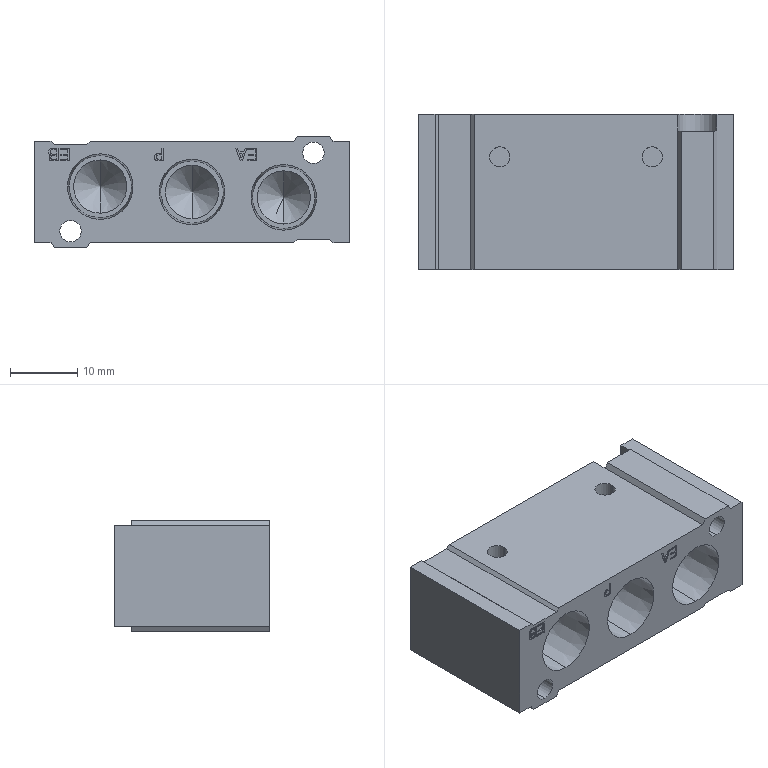Part | STEP file | 11-sy5120-5gz-01_sy51802block-V2.0-V2.011_20 | 1 solid | 176 faces | box 46.6 x 23 x 16.6 mm | volume 13080 mm3 | plane 121 | spline 22 | cylinder 21 | cone 12 | commonest cylinder face diameters 3 x8 7.9 x6 3.2 x4 5.8 x3